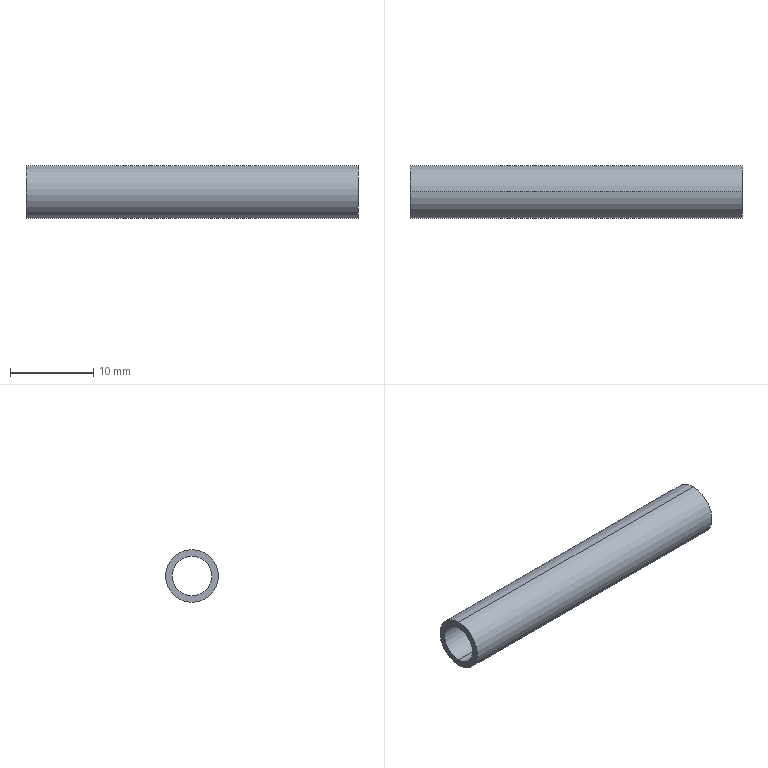Part | STEP file | copper tube 32_default_machined_ | 1 solid | 6 faces | box 40 x 6.35 x 6.35 mm | volume 557.947 mm3 | cylinder 4 | plane 2 | commonest cylinder face diameters 4.75 x2 6.35 x2
STEP:
#1=CARTESIAN_POINT('',(0.,0.,0.));
#2=DIRECTION('',(0.,0.,1.));
#3=DIRECTION('',(1.,0.,0.));
#4=AXIS2_PLACEMENT_3D('',#1,#2,#3);
#5=CARTESIAN_POINT('',(-40.,0.,-3.175));
#6=VERTEX_POINT('',#5);
#7=CARTESIAN_POINT('',(-40.,0.,3.175));
#8=VERTEX_POINT('',#7);
#9=CARTESIAN_POINT('',(-40.,0.,0.));
#10=DIRECTION('',(1.,0.,0.));
#11=DIRECTION('',(0.,0.,-1.));
#12=AXIS2_PLACEMENT_3D('',#9,#10,#11);
#13=CIRCLE('',#12,3.175);
#14=CARTESIAN_POINT('',(-40.,0.,0.));
#15=DIRECTION('',(1.,0.,0.));
#16=DIRECTION('',(0.,0.,-1.));
#17=AXIS2_PLACEMENT_3D('',#14,#15,#16);
#18=CYLINDRICAL_SURFACE('',#17,3.175);
#19=CARTESIAN_POINT('',(0.,0.));
#20=DIRECTION('',(1.,0.));
#21=VECTOR('',#20,1.);
#22=LINE('',#19,#21);
#23=(GEOMETRIC_REPRESENTATION_CONTEXT(2)PARAMETRIC_REPRESENTATION_CONTEXT()REPRESENTATION_CONTEXT('',''));
#24=DEFINITIONAL_REPRESENTATION('',(#22),#23);
#25=PCURVE('',#18,#24);
#26=CARTESIAN_POINT('',(-40.,0.,0.));
#27=DIRECTION('',(-1.,0.,0.));
#28=DIRECTION('',(0.,0.,1.));
#29=AXIS2_PLACEMENT_3D('',#26,#27,#28);
#30=PLANE('',#29);
#31=CARTESIAN_POINT('',(-3.175,0.));
#32=CARTESIAN_POINT('',(-3.175,5.499));
#33=CARTESIAN_POINT('',(1.587,2.75));
#34=CARTESIAN_POINT('',(6.35,0.));
#35=CARTESIAN_POINT('',(1.587,-2.75));
#36=CARTESIAN_POINT('',(-3.175,-5.499));
#37=CARTESIAN_POINT('',(-3.175,0.));
#38=(BOUNDED_CURVE()B_SPLINE_CURVE(2,(#31,#32,#33,#34,#35,#36,#37),.UNSPECIFIED.,.T.,.F.)B_SPLINE_CURVE_WITH_KNOTS((1,2,2,2,2,1),(-2.094,0.,2.094,4.189,6.283,8.378),.UNSPECIFIED.)CURVE()GEOMETRIC_REPRESENTATION_ITEM()RATIONAL_B_SPLINE_CURVE((1.,0.5,1.,0.5,1.,0.5,1.))REPRESENTATION_ITEM(''));
#39=(GEOMETRIC_REPRESENTATION_CONTEXT(2)PARAMETRIC_REPRESENTATION_CONTEXT()REPRESENTATION_CONTEXT('',''));
#40=DEFINITIONAL_REPRESENTATION('',(#38),#39);
#41=PCURVE('',#30,#40);
#42=SURFACE_CURVE('',#13,(#25,#41),.PCURVE_S1.);
#43=EDGE_CURVE('',#6,#8,#42,.T.);
#44=ORIENTED_EDGE('',*,*,#43,.T.);
#45=CARTESIAN_POINT('',(0.,0.,3.175));
#46=VERTEX_POINT('',#45);
#47=CARTESIAN_POINT('',(-40.,0.,3.175));
#48=DIRECTION('',(1.,0.,0.));
#49=VECTOR('',#48,1.);
#50=LINE('',#47,#49);
#51=CARTESIAN_POINT('',(3.142,0.));
#52=DIRECTION('',(0.,1.));
#53=VECTOR('',#52,1.);
#54=LINE('',#51,#53);
#55=(GEOMETRIC_REPRESENTATION_CONTEXT(2)PARAMETRIC_REPRESENTATION_CONTEXT()REPRESENTATION_CONTEXT('',''));
#56=DEFINITIONAL_REPRESENTATION('',(#54),#55);
#57=PCURVE('',#18,#56);
#58=CARTESIAN_POINT('',(-40.,0.,0.));
#59=DIRECTION('',(1.,0.,0.));
#60=DIRECTION('',(0.,0.,-1.));
#61=AXIS2_PLACEMENT_3D('',#58,#59,#60);
#62=CYLINDRICAL_SURFACE('',#61,3.175);
#63=CARTESIAN_POINT('',(3.142,0.));
#64=DIRECTION('',(0.,1.));
#65=VECTOR('',#64,1.);
#66=LINE('',#63,#65);
#67=(GEOMETRIC_REPRESENTATION_CONTEXT(2)PARAMETRIC_REPRESENTATION_CONTEXT()REPRESENTATION_CONTEXT('',''));
#68=DEFINITIONAL_REPRESENTATION('',(#66),#67);
#69=PCURVE('',#62,#68);
#70=SURFACE_CURVE('',#50,(#57,#69),.PCURVE_S1.);
#71=EDGE_CURVE('',#8,#46,#70,.T.);
#72=ORIENTED_EDGE('',*,*,#71,.T.);
#73=CARTESIAN_POINT('',(0.,0.,-3.175));
#74=VERTEX_POINT('',#73);
#75=CARTESIAN_POINT('',(0.,0.,0.));
#76=DIRECTION('',(-1.,0.,0.));
#77=DIRECTION('',(0.,0.,-1.));
#78=AXIS2_PLACEMENT_3D('',#75,#76,#77);
#79=CIRCLE('',#78,3.175);
#80=CARTESIAN_POINT('',(6.283,40.));
#81=DIRECTION('',(-1.,0.));
#82=VECTOR('',#81,1.);
#83=LINE('',#80,#82);
#84=(GEOMETRIC_REPRESENTATION_CONTEXT(2)PARAMETRIC_REPRESENTATION_CONTEXT()REPRESENTATION_CONTEXT('',''));
#85=DEFINITIONAL_REPRESENTATION('',(#83),#84);
#86=PCURVE('',#18,#85);
#87=CARTESIAN_POINT('',(0.,0.,0.));
#88=DIRECTION('',(-1.,0.,0.));
#89=DIRECTION('',(0.,0.,1.));
#90=AXIS2_PLACEMENT_3D('',#87,#88,#89);
#91=PLANE('',#90);
#92=CARTESIAN_POINT('',(0.,0.));
#93=DIRECTION('',(-1.,0.));
#94=AXIS2_PLACEMENT_2D('',#92,#93);
#95=CIRCLE('',#94,3.175);
#96=(GEOMETRIC_REPRESENTATION_CONTEXT(2)PARAMETRIC_REPRESENTATION_CONTEXT()REPRESENTATION_CONTEXT('',''));
#97=DEFINITIONAL_REPRESENTATION('',(#95),#96);
#98=PCURVE('',#91,#97);
#99=SURFACE_CURVE('',#79,(#86,#98),.PCURVE_S1.);
#100=EDGE_CURVE('',#46,#74,#99,.T.);
#101=ORIENTED_EDGE('',*,*,#100,.T.);
#102=CARTESIAN_POINT('',(-40.,0.,-3.175));
#103=DIRECTION('',(1.,0.,0.));
#104=VECTOR('',#103,1.);
#105=LINE('',#102,#104);
#106=CARTESIAN_POINT('',(0.,0.));
#107=DIRECTION('',(0.,1.));
#108=VECTOR('',#107,1.);
#109=LINE('',#106,#108);
#110=(GEOMETRIC_REPRESENTATION_CONTEXT(2)PARAMETRIC_REPRESENTATION_CONTEXT()REPRESENTATION_CONTEXT('',''));
#111=DEFINITIONAL_REPRESENTATION('',(#109),#110);
#112=PCURVE('',#18,#111);
#113=CARTESIAN_POINT('',(6.283,0.));
#114=DIRECTION('',(0.,1.));
#115=VECTOR('',#114,1.);
#116=LINE('',#113,#115);
#117=(GEOMETRIC_REPRESENTATION_CONTEXT(2)PARAMETRIC_REPRESENTATION_CONTEXT()REPRESENTATION_CONTEXT('',''));
#118=DEFINITIONAL_REPRESENTATION('',(#116),#117);
#119=PCURVE('',#62,#118);
#120=SURFACE_CURVE('',#105,(#112,#119),.PCURVE_S1.);
#121=EDGE_CURVE('',#6,#74,#120,.T.);
#122=ORIENTED_EDGE('',*,*,#121,.F.);
#123=EDGE_LOOP('',(#44,#72,#101,#122));
#124=FACE_BOUND('',#123,.T.);
#125=ADVANCED_FACE('',(#124),#18,.T.);
#126=CARTESIAN_POINT('',(-40.,0.,-2.375));
#127=VERTEX_POINT('',#126);
#128=CARTESIAN_POINT('',(0.,0.,-2.375));
#129=VERTEX_POINT('',#128);
#130=CARTESIAN_POINT('',(-40.,0.,-2.375));
#131=DIRECTION('',(1.,0.,0.));
#132=VECTOR('',#131,1.);
#133=LINE('',#130,#132);
#134=CARTESIAN_POINT('',(-40.,0.,0.));
#135=DIRECTION('',(1.,0.,0.));
#136=DIRECTION('',(0.,0.,-1.));
#137=AXIS2_PLACEMENT_3D('',#134,#135,#136);
#138=CYLINDRICAL_SURFACE('',#137,2.375);
#139=CARTESIAN_POINT('',(6.283,0.));
#140=DIRECTION('',(0.,1.));
#141=VECTOR('',#140,1.);
#142=LINE('',#139,#141);
#143=(GEOMETRIC_REPRESENTATION_CONTEXT(2)PARAMETRIC_REPRESENTATION_CONTEXT()REPRESENTATION_CONTEXT('',''));
#144=DEFINITIONAL_REPRESENTATION('',(#142),#143);
#145=PCURVE('',#138,#144);
#146=CARTESIAN_POINT('',(-40.,0.,0.));
#147=DIRECTION('',(1.,0.,0.));
#148=DIRECTION('',(0.,0.,-1.));
#149=AXIS2_PLACEMENT_3D('',#146,#147,#148);
#150=CYLINDRICAL_SURFACE('',#149,2.375);
#151=CARTESIAN_POINT('',(0.,0.));
#152=DIRECTION('',(0.,1.));
#153=VECTOR('',#152,1.);
#154=LINE('',#151,#153);
#155=(GEOMETRIC_REPRESENTATION_CONTEXT(2)PARAMETRIC_REPRESENTATION_CONTEXT()REPRESENTATION_CONTEXT('',''));
#156=DEFINITIONAL_REPRESENTATION('',(#154),#155);
#157=PCURVE('',#150,#156);
#158=SURFACE_CURVE('',#133,(#145,#157),.PCURVE_S1.);
#159=EDGE_CURVE('',#127,#129,#158,.T.);
#160=ORIENTED_EDGE('',*,*,#159,.T.);
#161=CARTESIAN_POINT('',(0.,0.,2.375));
#162=VERTEX_POINT('',#161);
#163=CARTESIAN_POINT('',(0.,0.,0.));
#164=DIRECTION('',(1.,0.,0.));
#165=DIRECTION('',(0.,0.,-1.));
#166=AXIS2_PLACEMENT_3D('',#163,#164,#165);
#167=CIRCLE('',#166,2.375);
#168=CARTESIAN_POINT('',(0.,40.));
#169=DIRECTION('',(1.,0.));
#170=VECTOR('',#169,1.);
#171=LINE('',#168,#170);
#172=(GEOMETRIC_REPRESENTATION_CONTEXT(2)PARAMETRIC_REPRESENTATION_CONTEXT()REPRESENTATION_CONTEXT('',''));
#173=DEFINITIONAL_REPRESENTATION('',(#171),#172);
#174=PCURVE('',#138,#173);
#175=CARTESIAN_POINT('',(-2.375,0.));
#176=CARTESIAN_POINT('',(-2.375,4.114));
#177=CARTESIAN_POINT('',(1.188,2.057));
#178=CARTESIAN_POINT('',(4.75,0.));
#179=CARTESIAN_POINT('',(1.188,-2.057));
#180=CARTESIAN_POINT('',(-2.375,-4.114));
#181=CARTESIAN_POINT('',(-2.375,0.));
#182=(BOUNDED_CURVE()B_SPLINE_CURVE(2,(#175,#176,#177,#178,#179,#180,#181),.UNSPECIFIED.,.T.,.F.)B_SPLINE_CURVE_WITH_KNOTS((1,2,2,2,2,1),(-2.094,0.,2.094,4.189,6.283,8.378),.UNSPECIFIED.)CURVE()GEOMETRIC_REPRESENTATION_ITEM()RATIONAL_B_SPLINE_CURVE((1.,0.5,1.,0.5,1.,0.5,1.))REPRESENTATION_ITEM(''));
#183=(GEOMETRIC_REPRESENTATION_CONTEXT(2)PARAMETRIC_REPRESENTATION_CONTEXT()REPRESENTATION_CONTEXT('',''));
#184=DEFINITIONAL_REPRESENTATION('',(#182),#183);
#185=PCURVE('',#91,#184);
#186=SURFACE_CURVE('',#167,(#174,#185),.PCURVE_S1.);
#187=EDGE_CURVE('',#162,#129,#186,.T.);
#188=ORIENTED_EDGE('',*,*,#187,.F.);
#189=CARTESIAN_POINT('',(-40.,0.,2.375));
#190=VERTEX_POINT('',#189);
#191=CARTESIAN_POINT('',(-40.,0.,2.375));
#192=DIRECTION('',(1.,0.,0.));
#193=VECTOR('',#192,1.);
#194=LINE('',#191,#193);
#195=CARTESIAN_POINT('',(3.142,0.));
#196=DIRECTION('',(0.,1.));
#197=VECTOR('',#196,1.);
#198=LINE('',#195,#197);
#199=(GEOMETRIC_REPRESENTATION_CONTEXT(2)PARAMETRIC_REPRESENTATION_CONTEXT()REPRESENTATION_CONTEXT('',''));
#200=DEFINITIONAL_REPRESENTATION('',(#198),#199);
#201=PCURVE('',#138,#200);
#202=CARTESIAN_POINT('',(3.142,0.));
#203=DIRECTION('',(0.,1.));
#204=VECTOR('',#203,1.);
#205=LINE('',#202,#204);
#206=(GEOMETRIC_REPRESENTATION_CONTEXT(2)PARAMETRIC_REPRESENTATION_CONTEXT()REPRESENTATION_CONTEXT('',''));
#207=DEFINITIONAL_REPRESENTATION('',(#205),#206);
#208=PCURVE('',#150,#207);
#209=SURFACE_CURVE('',#194,(#201,#208),.PCURVE_S1.);
#210=EDGE_CURVE('',#190,#162,#209,.T.);
#211=ORIENTED_EDGE('',*,*,#210,.F.);
#212=CARTESIAN_POINT('',(-40.,0.,0.));
#213=DIRECTION('',(1.,0.,0.));
#214=DIRECTION('',(0.,0.,-1.));
#215=AXIS2_PLACEMENT_3D('',#212,#213,#214);
#216=CIRCLE('',#215,2.375);
#217=CARTESIAN_POINT('',(0.,0.));
#218=DIRECTION('',(1.,0.));
#219=VECTOR('',#218,1.);
#220=LINE('',#217,#219);
#221=(GEOMETRIC_REPRESENTATION_CONTEXT(2)PARAMETRIC_REPRESENTATION_CONTEXT()REPRESENTATION_CONTEXT('',''));
#222=DEFINITIONAL_REPRESENTATION('',(#220),#221);
#223=PCURVE('',#138,#222);
#224=CARTESIAN_POINT('',(-2.375,0.));
#225=CARTESIAN_POINT('',(-2.375,4.114));
#226=CARTESIAN_POINT('',(1.188,2.057));
#227=CARTESIAN_POINT('',(4.75,0.));
#228=CARTESIAN_POINT('',(1.188,-2.057));
#229=CARTESIAN_POINT('',(-2.375,-4.114));
#230=CARTESIAN_POINT('',(-2.375,0.));
#231=(BOUNDED_CURVE()B_SPLINE_CURVE(2,(#224,#225,#226,#227,#228,#229,#230),.UNSPECIFIED.,.T.,.F.)B_SPLINE_CURVE_WITH_KNOTS((1,2,2,2,2,1),(-2.094,0.,2.094,4.189,6.283,8.378),.UNSPECIFIED.)CURVE()GEOMETRIC_REPRESENTATION_ITEM()RATIONAL_B_SPLINE_CURVE((1.,0.5,1.,0.5,1.,0.5,1.))REPRESENTATION_ITEM(''));
#232=(GEOMETRIC_REPRESENTATION_CONTEXT(2)PARAMETRIC_REPRESENTATION_CONTEXT()REPRESENTATION_CONTEXT('',''));
#233=DEFINITIONAL_REPRESENTATION('',(#231),#232);
#234=PCURVE('',#30,#233);
#235=SURFACE_CURVE('',#216,(#223,#234),.PCURVE_S1.);
#236=EDGE_CURVE('',#190,#127,#235,.T.);
#237=ORIENTED_EDGE('',*,*,#236,.T.);
#238=EDGE_LOOP('',(#160,#188,#211,#237));
#239=FACE_BOUND('',#238,.F.);
#240=ADVANCED_FACE('',(#239),#138,.F.);
#241=ORIENTED_EDGE('',*,*,#71,.F.);
#242=CARTESIAN_POINT('',(-40.,0.,0.));
#243=DIRECTION('',(1.,0.,0.));
#244=DIRECTION('',(0.,0.,-1.));
#245=AXIS2_PLACEMENT_3D('',#242,#243,#244);
#246=CIRCLE('',#245,3.175);
#247=CARTESIAN_POINT('',(0.,0.));
#248=DIRECTION('',(1.,0.));
#249=VECTOR('',#248,1.);
#250=LINE('',#247,#249);
#251=(GEOMETRIC_REPRESENTATION_CONTEXT(2)PARAMETRIC_REPRESENTATION_CONTEXT()REPRESENTATION_CONTEXT('',''));
#252=DEFINITIONAL_REPRESENTATION('',(#250),#251);
#253=PCURVE('',#62,#252);
#254=CARTESIAN_POINT('',(-3.175,0.));
#255=CARTESIAN_POINT('',(-3.175,5.499));
#256=CARTESIAN_POINT('',(1.587,2.75));
#257=CARTESIAN_POINT('',(6.35,0.));
#258=CARTESIAN_POINT('',(1.587,-2.75));
#259=CARTESIAN_POINT('',(-3.175,-5.499));
#260=CARTESIAN_POINT('',(-3.175,0.));
#261=(BOUNDED_CURVE()B_SPLINE_CURVE(2,(#254,#255,#256,#257,#258,#259,#260),.UNSPECIFIED.,.T.,.F.)B_SPLINE_CURVE_WITH_KNOTS((1,2,2,2,2,1),(-2.094,0.,2.094,4.189,6.283,8.378),.UNSPECIFIED.)CURVE()GEOMETRIC_REPRESENTATION_ITEM()RATIONAL_B_SPLINE_CURVE((1.,0.5,1.,0.5,1.,0.5,1.))REPRESENTATION_ITEM(''));
#262=(GEOMETRIC_REPRESENTATION_CONTEXT(2)PARAMETRIC_REPRESENTATION_CONTEXT()REPRESENTATION_CONTEXT('',''));
#263=DEFINITIONAL_REPRESENTATION('',(#261),#262);
#264=PCURVE('',#30,#263);
#265=SURFACE_CURVE('',#246,(#253,#264),.PCURVE_S1.);
#266=EDGE_CURVE('',#8,#6,#265,.T.);
#267=ORIENTED_EDGE('',*,*,#266,.T.);
#268=ORIENTED_EDGE('',*,*,#121,.T.);
#269=CARTESIAN_POINT('',(0.,0.,0.));
#270=DIRECTION('',(-1.,0.,0.));
#271=DIRECTION('',(0.,0.,-1.));
#272=AXIS2_PLACEMENT_3D('',#269,#270,#271);
#273=CIRCLE('',#272,3.175);
#274=CARTESIAN_POINT('',(6.283,40.));
#275=DIRECTION('',(-1.,0.));
#276=VECTOR('',#275,1.);
#277=LINE('',#274,#276);
#278=(GEOMETRIC_REPRESENTATION_CONTEXT(2)PARAMETRIC_REPRESENTATION_CONTEXT()REPRESENTATION_CONTEXT('',''));
#279=DEFINITIONAL_REPRESENTATION('',(#277),#278);
#280=PCURVE('',#62,#279);
#281=CARTESIAN_POINT('',(0.,0.));
#282=DIRECTION('',(-1.,0.));
#283=AXIS2_PLACEMENT_2D('',#281,#282);
#284=CIRCLE('',#283,3.175);
#285=(GEOMETRIC_REPRESENTATION_CONTEXT(2)PARAMETRIC_REPRESENTATION_CONTEXT()REPRESENTATION_CONTEXT('',''));
#286=DEFINITIONAL_REPRESENTATION('',(#284),#285);
#287=PCURVE('',#91,#286);
#288=SURFACE_CURVE('',#273,(#280,#287),.PCURVE_S1.);
#289=EDGE_CURVE('',#74,#46,#288,.T.);
#290=ORIENTED_EDGE('',*,*,#289,.T.);
#291=EDGE_LOOP('',(#241,#267,#268,#290));
#292=FACE_BOUND('',#291,.T.);
#293=ADVANCED_FACE('',(#292),#62,.T.);
#294=ORIENTED_EDGE('',*,*,#289,.F.);
#295=ORIENTED_EDGE('',*,*,#100,.F.);
#296=EDGE_LOOP('',(#294,#295));
#297=FACE_BOUND('',#296,.T.);
#298=CARTESIAN_POINT('',(0.,0.,0.));
#299=DIRECTION('',(1.,0.,0.));
#300=DIRECTION('',(0.,0.,-1.));
#301=AXIS2_PLACEMENT_3D('',#298,#299,#300);
#302=CIRCLE('',#301,2.375);
#303=CARTESIAN_POINT('',(-2.375,0.));
#304=CARTESIAN_POINT('',(-2.375,4.114));
#305=CARTESIAN_POINT('',(1.188,2.057));
#306=CARTESIAN_POINT('',(4.75,0.));
#307=CARTESIAN_POINT('',(1.188,-2.057));
#308=CARTESIAN_POINT('',(-2.375,-4.114));
#309=CARTESIAN_POINT('',(-2.375,0.));
#310=(BOUNDED_CURVE()B_SPLINE_CURVE(2,(#303,#304,#305,#306,#307,#308,#309),.UNSPECIFIED.,.T.,.F.)B_SPLINE_CURVE_WITH_KNOTS((1,2,2,2,2,1),(-2.094,0.,2.094,4.189,6.283,8.378),.UNSPECIFIED.)CURVE()GEOMETRIC_REPRESENTATION_ITEM()RATIONAL_B_SPLINE_CURVE((1.,0.5,1.,0.5,1.,0.5,1.))REPRESENTATION_ITEM(''));
#311=(GEOMETRIC_REPRESENTATION_CONTEXT(2)PARAMETRIC_REPRESENTATION_CONTEXT()REPRESENTATION_CONTEXT('',''));
#312=DEFINITIONAL_REPRESENTATION('',(#310),#311);
#313=PCURVE('',#91,#312);
#314=CARTESIAN_POINT('',(0.,40.));
#315=DIRECTION('',(1.,0.));
#316=VECTOR('',#315,1.);
#317=LINE('',#314,#316);
#318=(GEOMETRIC_REPRESENTATION_CONTEXT(2)PARAMETRIC_REPRESENTATION_CONTEXT()REPRESENTATION_CONTEXT('',''));
#319=DEFINITIONAL_REPRESENTATION('',(#317),#318);
#320=PCURVE('',#150,#319);
#321=SURFACE_CURVE('',#302,(#313,#320),.PCURVE_S1.);
#322=EDGE_CURVE('',#129,#162,#321,.T.);
#323=ORIENTED_EDGE('',*,*,#322,.F.);
#324=ORIENTED_EDGE('',*,*,#187,.F.);
#325=EDGE_LOOP('',(#323,#324));
#326=FACE_BOUND('',#325,.T.);
#327=ADVANCED_FACE('',(#297,#326),#91,.F.);
#328=ORIENTED_EDGE('',*,*,#43,.F.);
#329=ORIENTED_EDGE('',*,*,#266,.F.);
#330=EDGE_LOOP('',(#328,#329));
#331=FACE_BOUND('',#330,.T.);
#332=CARTESIAN_POINT('',(-40.,0.,0.));
#333=DIRECTION('',(1.,0.,0.));
#334=DIRECTION('',(0.,0.,-1.));
#335=AXIS2_PLACEMENT_3D('',#332,#333,#334);
#336=CIRCLE('',#335,2.375);
#337=CARTESIAN_POINT('',(-2.375,0.));
#338=CARTESIAN_POINT('',(-2.375,4.114));
#339=CARTESIAN_POINT('',(1.188,2.057));
#340=CARTESIAN_POINT('',(4.75,0.));
#341=CARTESIAN_POINT('',(1.188,-2.057));
#342=CARTESIAN_POINT('',(-2.375,-4.114));
#343=CARTESIAN_POINT('',(-2.375,0.));
#344=(BOUNDED_CURVE()B_SPLINE_CURVE(2,(#337,#338,#339,#340,#341,#342,#343),.UNSPECIFIED.,.T.,.F.)B_SPLINE_CURVE_WITH_KNOTS((1,2,2,2,2,1),(-2.094,0.,2.094,4.189,6.283,8.378),.UNSPECIFIED.)CURVE()GEOMETRIC_REPRESENTATION_ITEM()RATIONAL_B_SPLINE_CURVE((1.,0.5,1.,0.5,1.,0.5,1.))REPRESENTATION_ITEM(''));
#345=(GEOMETRIC_REPRESENTATION_CONTEXT(2)PARAMETRIC_REPRESENTATION_CONTEXT()REPRESENTATION_CONTEXT('',''));
#346=DEFINITIONAL_REPRESENTATION('',(#344),#345);
#347=PCURVE('',#30,#346);
#348=CARTESIAN_POINT('',(0.,0.));
#349=DIRECTION('',(1.,0.));
#350=VECTOR('',#349,1.);
#351=LINE('',#348,#350);
#352=(GEOMETRIC_REPRESENTATION_CONTEXT(2)PARAMETRIC_REPRESENTATION_CONTEXT()REPRESENTATION_CONTEXT('',''));
#353=DEFINITIONAL_REPRESENTATION('',(#351),#352);
#354=PCURVE('',#150,#353);
#355=SURFACE_CURVE('',#336,(#347,#354),.PCURVE_S1.);
#356=EDGE_CURVE('',#127,#190,#355,.T.);
#357=ORIENTED_EDGE('',*,*,#356,.T.);
#358=ORIENTED_EDGE('',*,*,#236,.T.);
#359=EDGE_LOOP('',(#357,#358));
#360=FACE_BOUND('',#359,.T.);
#361=ADVANCED_FACE('',(#331,#360),#30,.T.);
#362=ORIENTED_EDGE('',*,*,#322,.F.);
#363=ORIENTED_EDGE('',*,*,#159,.F.);
#364=ORIENTED_EDGE('',*,*,#356,.T.);
#365=ORIENTED_EDGE('',*,*,#210,.T.);
#366=EDGE_LOOP('',(#362,#363,#364,#365));
#367=FACE_BOUND('',#366,.F.);
#368=ADVANCED_FACE('',(#367),#150,.F.);
#369=CLOSED_SHELL('',(#125,#240,#293,#327,#361,#368));
#370=MANIFOLD_SOLID_BREP('',#369);
#371=(LENGTH_UNIT()NAMED_UNIT(*)SI_UNIT(.MILLI.,.METRE.));
#372=UNCERTAINTY_MEASURE_WITH_UNIT(LENGTH_MEASURE(0.0000001),#371,'','');
#373=(NAMED_UNIT(*)PLANE_ANGLE_UNIT()SI_UNIT($,.RADIAN.));
#374=(NAMED_UNIT(*)SI_UNIT($,.STERADIAN.)SOLID_ANGLE_UNIT());
#375=(GEOMETRIC_REPRESENTATION_CONTEXT(3)GLOBAL_UNCERTAINTY_ASSIGNED_CONTEXT((#372))GLOBAL_UNIT_ASSIGNED_CONTEXT((#371,#373,#374))REPRESENTATION_CONTEXT('',''));
#376=ADVANCED_BREP_SHAPE_REPRESENTATION('',(#4,#370),#375);